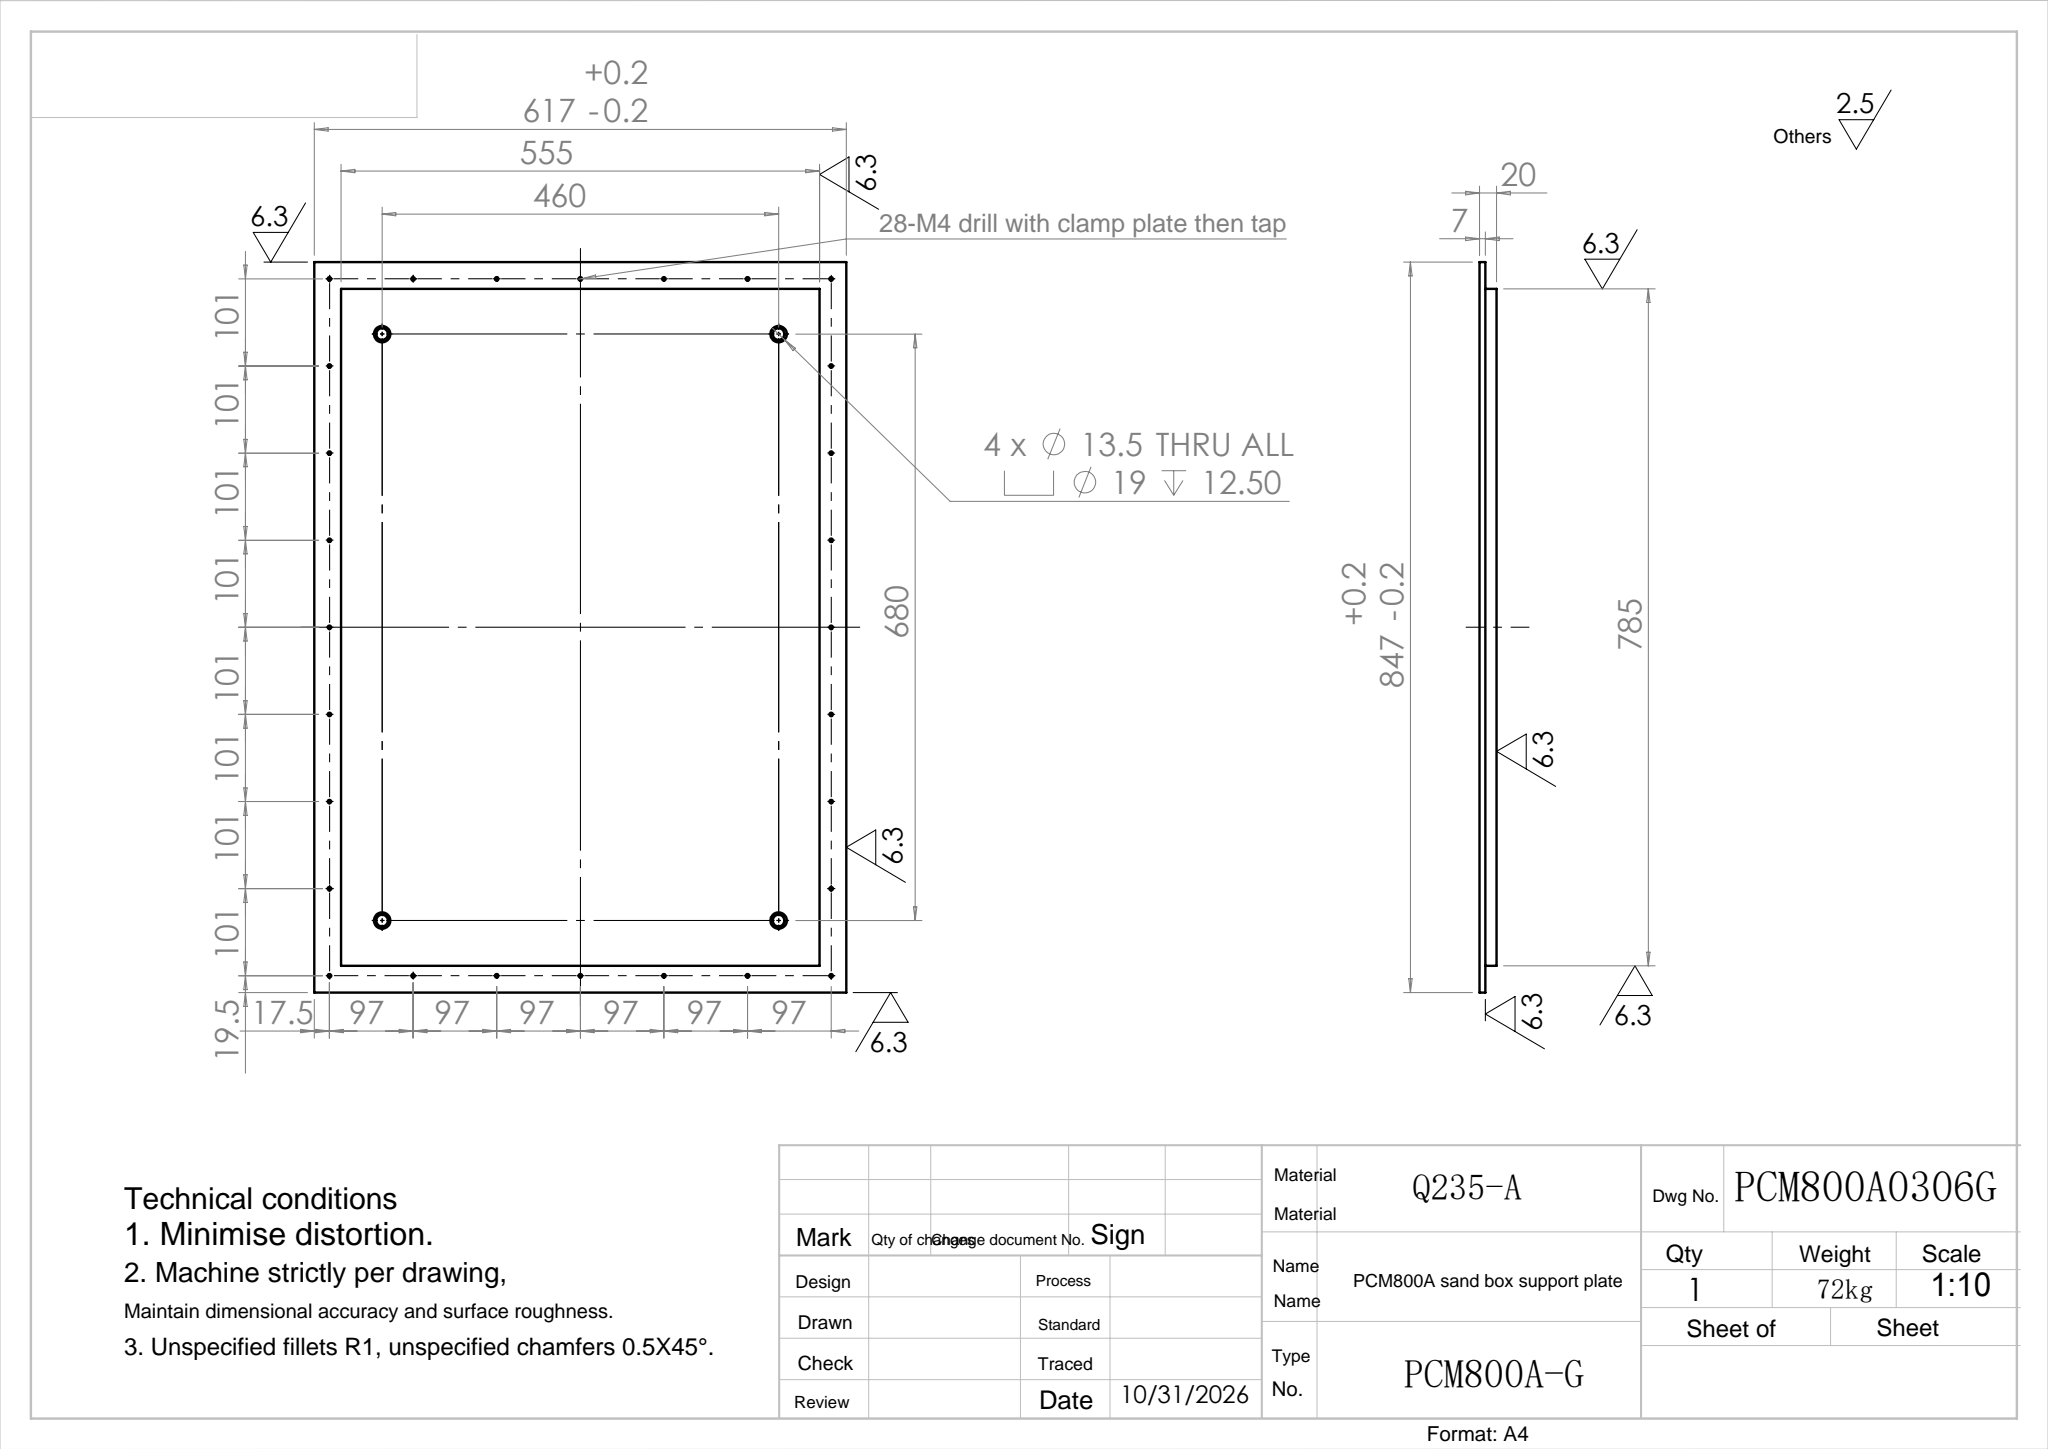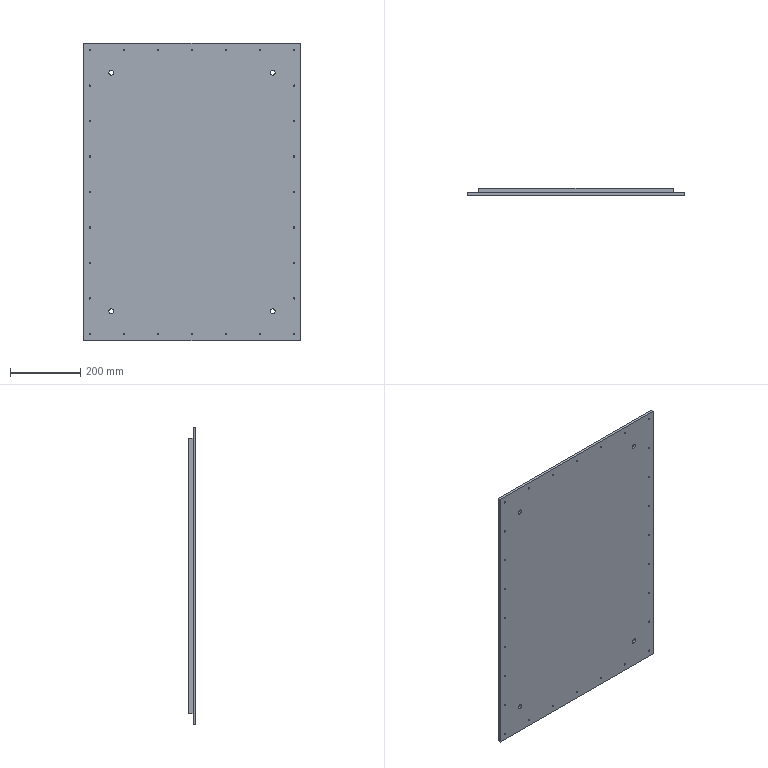Part | SolidWorks | features LPattern 3, Cut 2, HoleWzd 2, ICE 2, 3DProfileFeature 1, Extrusion 1 | 1 solid | 87 faces | box 617 x 20 x 847 mm | volume 9301034 mm3 | cylinder 72 | plane 15 | commonest cylinder face diameters 4 x56 13.5 x8 19 x8